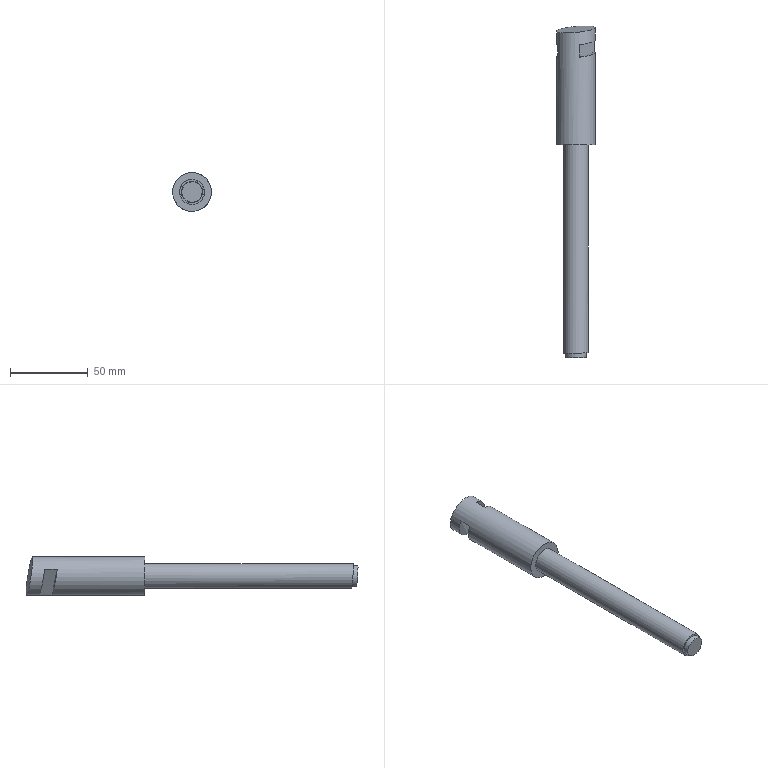Part | STEP file | solid 155 | 1 solid | 13 faces | box 25 x 214.101 x 25 mm | volume 62890 mm3 | plane 8 | spline 3 | cylinder 2 | commonest cylinder face diameters 16 x1 25 x1